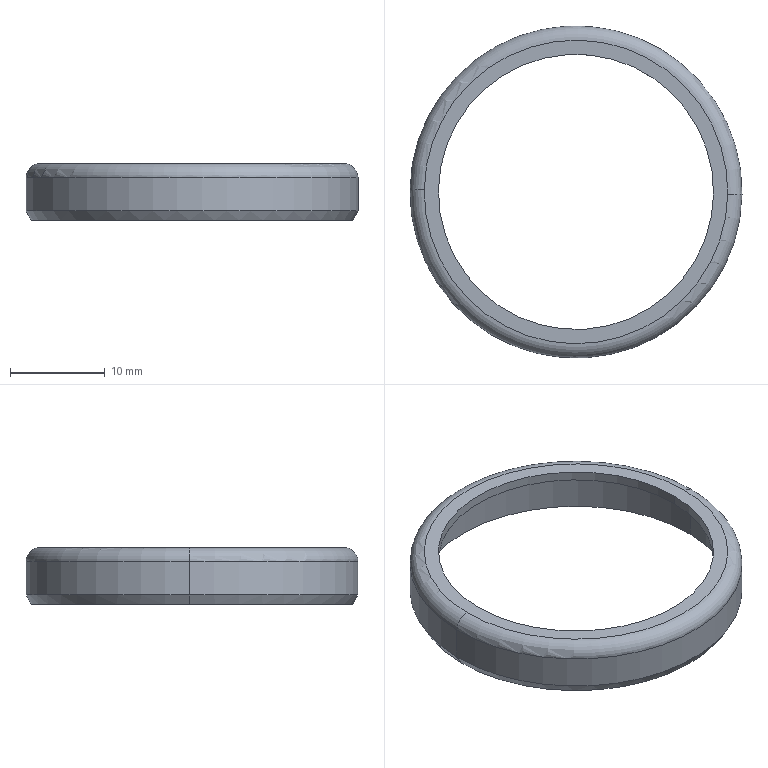Part | SolidWorks | features BaseBody 1 | 1 solid | 15 faces | box 35 x 35 x 6 mm | volume 627.231 mm3 | cylinder 6 | torus 4 | plane 3 | cone 2 | commonest cylinder face diameters 29 x2 33.5 x2 35 x2
STEP:
#1=CARTESIAN_POINT('',(-61.384,-49.853,89.25));
#2=VERTEX_POINT('',#1);
#3=CARTESIAN_POINT('',(-27.542,-50.354,89.25));
#4=VERTEX_POINT('',#3);
#5=CARTESIAN_POINT('',(-44.463,-50.104,89.25));
#6=DIRECTION('',(0.,0.,-1.));
#7=DIRECTION('',(-0.9999,0.01482,0.));
#8=AXIS2_PLACEMENT_3D('',#5,#6,#7);
#9=CIRCLE('',#8,16.923);
#10=EDGE_CURVE('',#2,#4,#9,.T.);
#11=ORIENTED_EDGE('',*,*,#10,.F.);
#12=CARTESIAN_POINT('',(-61.961,-49.845,90.25));
#13=VERTEX_POINT('',#12);
#14=CARTESIAN_POINT('',(-61.961,-49.845,90.25));
#15=DIRECTION('',(-0.4999,0.007408,0.866));
#16=VECTOR('',#15,1000.);
#17=LINE('',#14,#16);
#18=EDGE_CURVE('',#2,#13,#17,.T.);
#19=ORIENTED_EDGE('',*,*,#18,.T.);
#20=CARTESIAN_POINT('',(-26.965,-50.363,90.25));
#21=VERTEX_POINT('',#20);
#22=CARTESIAN_POINT('',(-44.463,-50.104,90.25));
#23=DIRECTION('',(0.,0.,-1.));
#24=DIRECTION('',(-0.9999,0.01482,0.));
#25=AXIS2_PLACEMENT_3D('',#22,#23,#24);
#26=CIRCLE('',#25,17.5);
#27=EDGE_CURVE('',#13,#21,#26,.T.);
#28=ORIENTED_EDGE('',*,*,#27,.T.);
#29=CARTESIAN_POINT('',(-26.965,-50.363,90.25));
#30=DIRECTION('',(0.4999,-0.007408,0.866));
#31=VECTOR('',#30,1000.);
#32=LINE('',#29,#31);
#33=EDGE_CURVE('',#4,#21,#32,.T.);
#34=ORIENTED_EDGE('',*,*,#33,.F.);
#35=EDGE_LOOP('',(#11,#19,#28,#34));
#36=FACE_OUTER_BOUND('',#35,.T.);
#37=CARTESIAN_POINT('',(-44.463,-50.104,90.25));
#38=DIRECTION('',(0.,0.,1.));
#39=DIRECTION('',(0.9999,-0.01482,0.));
#40=AXIS2_PLACEMENT_3D('',#37,#38,#39);
#41=CONICAL_SURFACE('',#40,17.5,0.5236);
#42=ADVANCED_FACE('',(#36),#41,.T.);
#43=CARTESIAN_POINT('',(-27.715,-50.352,93.75));
#44=VERTEX_POINT('',#43);
#45=CARTESIAN_POINT('',(-61.211,-49.856,93.75));
#46=VERTEX_POINT('',#45);
#47=CARTESIAN_POINT('',(-44.463,-50.104,93.75));
#48=DIRECTION('',(0.,0.,-1.));
#49=DIRECTION('',(-0.9999,0.01482,0.));
#50=AXIS2_PLACEMENT_3D('',#47,#48,#49);
#51=CIRCLE('',#50,16.75);
#52=EDGE_CURVE('',#44,#46,#51,.T.);
#53=ORIENTED_EDGE('',*,*,#52,.F.);
#54=CARTESIAN_POINT('',(-27.715,-50.352,89.25));
#55=VERTEX_POINT('',#54);
#56=CARTESIAN_POINT('',(-27.715,-50.352,89.25));
#57=DIRECTION('',(0.,0.,-1.));
#58=VECTOR('',#57,1000.);
#59=LINE('',#56,#58);
#60=EDGE_CURVE('',#44,#55,#59,.T.);
#61=ORIENTED_EDGE('',*,*,#60,.T.);
#62=CARTESIAN_POINT('',(-61.211,-49.856,89.25));
#63=VERTEX_POINT('',#62);
#64=CARTESIAN_POINT('',(-44.463,-50.104,89.25));
#65=DIRECTION('',(0.,0.,-1.));
#66=DIRECTION('',(-0.9999,0.01482,0.));
#67=AXIS2_PLACEMENT_3D('',#64,#65,#66);
#68=CIRCLE('',#67,16.75);
#69=EDGE_CURVE('',#55,#63,#68,.T.);
#70=ORIENTED_EDGE('',*,*,#69,.T.);
#71=CARTESIAN_POINT('',(-61.211,-49.856,89.25));
#72=DIRECTION('',(0.,0.,-1.));
#73=VECTOR('',#72,1000.);
#74=LINE('',#71,#73);
#75=EDGE_CURVE('',#46,#63,#74,.T.);
#76=ORIENTED_EDGE('',*,*,#75,.F.);
#77=EDGE_LOOP('',(#53,#61,#70,#76));
#78=FACE_OUTER_BOUND('',#77,.T.);
#79=CARTESIAN_POINT('',(-44.463,-50.104,89.25));
#80=DIRECTION('',(0.,0.,-1.));
#81=DIRECTION('',(-0.9999,0.01482,0.));
#82=AXIS2_PLACEMENT_3D('',#79,#80,#81);
#83=CYLINDRICAL_SURFACE('',#82,16.75);
#84=ADVANCED_FACE('',(#78),#83,.F.);
#85=CARTESIAN_POINT('',(-28.215,-50.345,94.25));
#86=VERTEX_POINT('',#85);
#87=CARTESIAN_POINT('',(-60.711,-49.863,94.25));
#88=VERTEX_POINT('',#87);
#89=CARTESIAN_POINT('',(-44.463,-50.104,94.25));
#90=DIRECTION('',(0.,0.,-1.));
#91=DIRECTION('',(-0.9999,0.01482,0.));
#92=AXIS2_PLACEMENT_3D('',#89,#90,#91);
#93=CIRCLE('',#92,16.25);
#94=EDGE_CURVE('',#86,#88,#93,.T.);
#95=ORIENTED_EDGE('',*,*,#94,.F.);
#96=CARTESIAN_POINT('',(-28.215,-50.345,93.75));
#97=DIRECTION('',(0.01482,0.9999,0.));
#98=DIRECTION('',(-0.9999,0.01482,0.));
#99=AXIS2_PLACEMENT_3D('',#96,#97,#98);
#100=CIRCLE('',#99,0.5);
#101=EDGE_CURVE('',#86,#44,#100,.T.);
#102=ORIENTED_EDGE('',*,*,#101,.T.);
#103=ORIENTED_EDGE('',*,*,#52,.T.);
#104=CARTESIAN_POINT('',(-60.711,-49.863,93.75));
#105=DIRECTION('',(-0.01482,-0.9999,0.));
#106=DIRECTION('',(0.9999,-0.01482,0.));
#107=AXIS2_PLACEMENT_3D('',#104,#105,#106);
#108=CIRCLE('',#107,0.5);
#109=EDGE_CURVE('',#88,#46,#108,.T.);
#110=ORIENTED_EDGE('',*,*,#109,.F.);
#111=EDGE_LOOP('',(#95,#102,#103,#110));
#112=FACE_OUTER_BOUND('',#111,.T.);
#113=CARTESIAN_POINT('',(-44.463,-50.104,93.75));
#114=DIRECTION('',(0.,0.,-1.));
#115=DIRECTION('',(-0.9999,0.01482,0.));
#116=AXIS2_PLACEMENT_3D('',#113,#114,#115);
#117=TOROIDAL_SURFACE('',#116,16.25,0.5);
#118=ADVANCED_FACE('',(#112),#117,.F.);
#119=CARTESIAN_POINT('',(-29.964,-50.319,95.25));
#120=VERTEX_POINT('',#119);
#121=CARTESIAN_POINT('',(-58.961,-49.889,95.25));
#122=VERTEX_POINT('',#121);
#123=CARTESIAN_POINT('',(-44.463,-50.104,95.25));
#124=DIRECTION('',(0.,0.,-1.));
#125=DIRECTION('',(-0.9999,0.01482,0.));
#126=AXIS2_PLACEMENT_3D('',#123,#124,#125);
#127=CIRCLE('',#126,14.5);
#128=EDGE_CURVE('',#120,#122,#127,.T.);
#129=ORIENTED_EDGE('',*,*,#128,.F.);
#130=CARTESIAN_POINT('',(-29.964,-50.319,94.25));
#131=VERTEX_POINT('',#130);
#132=CARTESIAN_POINT('',(-29.964,-50.319,89.25));
#133=DIRECTION('',(0.,0.,-1.));
#134=VECTOR('',#133,1000.);
#135=LINE('',#132,#134);
#136=EDGE_CURVE('',#120,#131,#135,.T.);
#137=ORIENTED_EDGE('',*,*,#136,.T.);
#138=CARTESIAN_POINT('',(-58.961,-49.889,94.25));
#139=VERTEX_POINT('',#138);
#140=CARTESIAN_POINT('',(-44.463,-50.104,94.25));
#141=DIRECTION('',(0.,0.,-1.));
#142=DIRECTION('',(-0.9999,0.01482,0.));
#143=AXIS2_PLACEMENT_3D('',#140,#141,#142);
#144=CIRCLE('',#143,14.5);
#145=EDGE_CURVE('',#131,#139,#144,.T.);
#146=ORIENTED_EDGE('',*,*,#145,.T.);
#147=CARTESIAN_POINT('',(-58.961,-49.889,89.25));
#148=DIRECTION('',(0.,0.,-1.));
#149=VECTOR('',#148,1000.);
#150=LINE('',#147,#149);
#151=EDGE_CURVE('',#122,#139,#150,.T.);
#152=ORIENTED_EDGE('',*,*,#151,.F.);
#153=EDGE_LOOP('',(#129,#137,#146,#152));
#154=FACE_OUTER_BOUND('',#153,.T.);
#155=CARTESIAN_POINT('',(-44.463,-50.104,89.25));
#156=DIRECTION('',(0.,0.,-1.));
#157=DIRECTION('',(-0.9999,0.01482,0.));
#158=AXIS2_PLACEMENT_3D('',#155,#156,#157);
#159=CYLINDRICAL_SURFACE('',#158,14.5);
#160=ADVANCED_FACE('',(#154),#159,.F.);
#161=CARTESIAN_POINT('',(-60.461,-49.867,95.25));
#162=VERTEX_POINT('',#161);
#163=CARTESIAN_POINT('',(-28.465,-50.341,95.25));
#164=VERTEX_POINT('',#163);
#165=CARTESIAN_POINT('',(-44.463,-50.104,95.25));
#166=DIRECTION('',(0.,0.,-1.));
#167=DIRECTION('',(-0.9999,0.01482,0.));
#168=AXIS2_PLACEMENT_3D('',#165,#166,#167);
#169=CIRCLE('',#168,16.);
#170=EDGE_CURVE('',#162,#164,#169,.T.);
#171=ORIENTED_EDGE('',*,*,#170,.T.);
#172=CARTESIAN_POINT('',(-26.965,-50.363,93.75));
#173=VERTEX_POINT('',#172);
#174=CARTESIAN_POINT('',(-28.465,-50.341,93.75));
#175=DIRECTION('',(0.01482,0.9999,0.));
#176=DIRECTION('',(-0.9999,0.01482,0.));
#177=AXIS2_PLACEMENT_3D('',#174,#175,#176);
#178=CIRCLE('',#177,1.5);
#179=EDGE_CURVE('',#164,#173,#178,.T.);
#180=ORIENTED_EDGE('',*,*,#179,.T.);
#181=CARTESIAN_POINT('',(-61.961,-49.845,93.75));
#182=VERTEX_POINT('',#181);
#183=CARTESIAN_POINT('',(-44.463,-50.104,93.75));
#184=DIRECTION('',(0.,0.,-1.));
#185=DIRECTION('',(-0.9999,0.01482,0.));
#186=AXIS2_PLACEMENT_3D('',#183,#184,#185);
#187=CIRCLE('',#186,17.5);
#188=EDGE_CURVE('',#182,#173,#187,.T.);
#189=ORIENTED_EDGE('',*,*,#188,.F.);
#190=CARTESIAN_POINT('',(-60.461,-49.867,93.75));
#191=DIRECTION('',(-0.01482,-0.9999,0.));
#192=DIRECTION('',(0.9999,-0.01482,0.));
#193=AXIS2_PLACEMENT_3D('',#190,#191,#192);
#194=CIRCLE('',#193,1.5);
#195=EDGE_CURVE('',#162,#182,#194,.T.);
#196=ORIENTED_EDGE('',*,*,#195,.F.);
#197=EDGE_LOOP('',(#171,#180,#189,#196));
#198=FACE_OUTER_BOUND('',#197,.T.);
#199=CARTESIAN_POINT('',(-44.463,-50.104,93.75));
#200=DIRECTION('',(0.,0.,-1.));
#201=DIRECTION('',(-0.9999,0.01482,0.));
#202=AXIS2_PLACEMENT_3D('',#199,#200,#201);
#203=TOROIDAL_SURFACE('',#202,16.,1.5);
#204=ADVANCED_FACE('',(#198),#203,.T.);
#205=ORIENTED_EDGE('',*,*,#188,.T.);
#206=CARTESIAN_POINT('',(-26.965,-50.363,89.25));
#207=DIRECTION('',(0.,0.,-1.));
#208=VECTOR('',#207,1000.);
#209=LINE('',#206,#208);
#210=EDGE_CURVE('',#173,#21,#209,.T.);
#211=ORIENTED_EDGE('',*,*,#210,.T.);
#212=ORIENTED_EDGE('',*,*,#27,.F.);
#213=CARTESIAN_POINT('',(-61.961,-49.845,89.25));
#214=DIRECTION('',(0.,0.,-1.));
#215=VECTOR('',#214,1000.);
#216=LINE('',#213,#215);
#217=EDGE_CURVE('',#182,#13,#216,.T.);
#218=ORIENTED_EDGE('',*,*,#217,.F.);
#219=EDGE_LOOP('',(#205,#211,#212,#218));
#220=FACE_OUTER_BOUND('',#219,.T.);
#221=CARTESIAN_POINT('',(-44.463,-50.104,89.25));
#222=DIRECTION('',(0.,0.,-1.));
#223=DIRECTION('',(-0.9999,0.01482,0.));
#224=AXIS2_PLACEMENT_3D('',#221,#222,#223);
#225=CYLINDRICAL_SURFACE('',#224,17.5);
#226=ADVANCED_FACE('',(#220),#225,.T.);
#227=ORIENTED_EDGE('',*,*,#210,.F.);
#228=CARTESIAN_POINT('',(-44.463,-50.104,93.75));
#229=DIRECTION('',(0.,0.,-1.));
#230=DIRECTION('',(-0.9999,0.01482,0.));
#231=AXIS2_PLACEMENT_3D('',#228,#229,#230);
#232=CIRCLE('',#231,17.5);
#233=EDGE_CURVE('',#173,#182,#232,.T.);
#234=ORIENTED_EDGE('',*,*,#233,.T.);
#235=ORIENTED_EDGE('',*,*,#217,.T.);
#236=CARTESIAN_POINT('',(-44.463,-50.104,90.25));
#237=DIRECTION('',(0.,0.,-1.));
#238=DIRECTION('',(-0.9999,0.01482,0.));
#239=AXIS2_PLACEMENT_3D('',#236,#237,#238);
#240=CIRCLE('',#239,17.5);
#241=EDGE_CURVE('',#21,#13,#240,.T.);
#242=ORIENTED_EDGE('',*,*,#241,.F.);
#243=EDGE_LOOP('',(#227,#234,#235,#242));
#244=FACE_OUTER_BOUND('',#243,.T.);
#245=CARTESIAN_POINT('',(-44.463,-50.104,89.25));
#246=DIRECTION('',(0.,0.,-1.));
#247=DIRECTION('',(-0.9999,0.01482,0.));
#248=AXIS2_PLACEMENT_3D('',#245,#246,#247);
#249=CYLINDRICAL_SURFACE('',#248,17.5);
#250=ADVANCED_FACE('',(#244),#249,.T.);
#251=ORIENTED_EDGE('',*,*,#179,.F.);
#252=CARTESIAN_POINT('',(-44.463,-50.104,95.25));
#253=DIRECTION('',(0.,0.,-1.));
#254=DIRECTION('',(-0.9999,0.01482,0.));
#255=AXIS2_PLACEMENT_3D('',#252,#253,#254);
#256=CIRCLE('',#255,16.);
#257=EDGE_CURVE('',#164,#162,#256,.T.);
#258=ORIENTED_EDGE('',*,*,#257,.T.);
#259=ORIENTED_EDGE('',*,*,#195,.T.);
#260=ORIENTED_EDGE('',*,*,#233,.F.);
#261=EDGE_LOOP('',(#251,#258,#259,#260));
#262=FACE_OUTER_BOUND('',#261,.T.);
#263=CARTESIAN_POINT('',(-44.463,-50.104,93.75));
#264=DIRECTION('',(0.,0.,-1.));
#265=DIRECTION('',(-0.9999,0.01482,0.));
#266=AXIS2_PLACEMENT_3D('',#263,#264,#265);
#267=TOROIDAL_SURFACE('',#266,16.,1.5);
#268=ADVANCED_FACE('',(#262),#267,.T.);
#269=CARTESIAN_POINT('',(-44.463,-50.104,95.25));
#270=DIRECTION('',(0.,0.,-1.));
#271=DIRECTION('',(-0.9999,0.01482,0.));
#272=AXIS2_PLACEMENT_3D('',#269,#270,#271);
#273=CIRCLE('',#272,14.5);
#274=EDGE_CURVE('',#122,#120,#273,.T.);
#275=ORIENTED_EDGE('',*,*,#274,.T.);
#276=ORIENTED_EDGE('',*,*,#128,.T.);
#277=EDGE_LOOP('',(#275,#276));
#278=FACE_BOUND('',#277,.T.);
#279=ORIENTED_EDGE('',*,*,#170,.F.);
#280=ORIENTED_EDGE('',*,*,#257,.F.);
#281=EDGE_LOOP('',(#279,#280));
#282=FACE_OUTER_BOUND('',#281,.T.);
#283=CARTESIAN_POINT('',(-44.226,-34.106,95.25));
#284=DIRECTION('',(0.,0.,-1.));
#285=DIRECTION('',(-1.,0.,0.));
#286=AXIS2_PLACEMENT_3D('',#283,#284,#285);
#287=PLANE('',#286);
#288=ADVANCED_FACE('',(#278,#282),#287,.F.);
#289=ORIENTED_EDGE('',*,*,#136,.F.);
#290=ORIENTED_EDGE('',*,*,#274,.F.);
#291=ORIENTED_EDGE('',*,*,#151,.T.);
#292=CARTESIAN_POINT('',(-44.463,-50.104,94.25));
#293=DIRECTION('',(0.,0.,-1.));
#294=DIRECTION('',(-0.9999,0.01482,0.));
#295=AXIS2_PLACEMENT_3D('',#292,#293,#294);
#296=CIRCLE('',#295,14.5);
#297=EDGE_CURVE('',#139,#131,#296,.T.);
#298=ORIENTED_EDGE('',*,*,#297,.T.);
#299=EDGE_LOOP('',(#289,#290,#291,#298));
#300=FACE_OUTER_BOUND('',#299,.T.);
#301=CARTESIAN_POINT('',(-44.463,-50.104,89.25));
#302=DIRECTION('',(0.,0.,-1.));
#303=DIRECTION('',(-0.9999,0.01482,0.));
#304=AXIS2_PLACEMENT_3D('',#301,#302,#303);
#305=CYLINDRICAL_SURFACE('',#304,14.5);
#306=ADVANCED_FACE('',(#300),#305,.F.);
#307=CARTESIAN_POINT('',(-44.463,-50.104,94.25));
#308=DIRECTION('',(0.,0.,-1.));
#309=DIRECTION('',(-0.9999,0.01482,0.));
#310=AXIS2_PLACEMENT_3D('',#307,#308,#309);
#311=CIRCLE('',#310,16.25);
#312=EDGE_CURVE('',#88,#86,#311,.T.);
#313=ORIENTED_EDGE('',*,*,#312,.T.);
#314=ORIENTED_EDGE('',*,*,#94,.T.);
#315=EDGE_LOOP('',(#313,#314));
#316=FACE_OUTER_BOUND('',#315,.T.);
#317=ORIENTED_EDGE('',*,*,#297,.F.);
#318=ORIENTED_EDGE('',*,*,#145,.F.);
#319=EDGE_LOOP('',(#317,#318));
#320=FACE_BOUND('',#319,.T.);
#321=CARTESIAN_POINT('',(-44.248,-35.605,94.25));
#322=DIRECTION('',(0.,0.,1.));
#323=DIRECTION('',(1.,0.,0.));
#324=AXIS2_PLACEMENT_3D('',#321,#322,#323);
#325=PLANE('',#324);
#326=ADVANCED_FACE('',(#316,#320),#325,.F.);
#327=ORIENTED_EDGE('',*,*,#101,.F.);
#328=ORIENTED_EDGE('',*,*,#312,.F.);
#329=ORIENTED_EDGE('',*,*,#109,.T.);
#330=CARTESIAN_POINT('',(-44.463,-50.104,93.75));
#331=DIRECTION('',(0.,0.,-1.));
#332=DIRECTION('',(-0.9999,0.01482,0.));
#333=AXIS2_PLACEMENT_3D('',#330,#331,#332);
#334=CIRCLE('',#333,16.75);
#335=EDGE_CURVE('',#46,#44,#334,.T.);
#336=ORIENTED_EDGE('',*,*,#335,.T.);
#337=EDGE_LOOP('',(#327,#328,#329,#336));
#338=FACE_OUTER_BOUND('',#337,.T.);
#339=CARTESIAN_POINT('',(-44.463,-50.104,93.75));
#340=DIRECTION('',(0.,0.,-1.));
#341=DIRECTION('',(-0.9999,0.01482,0.));
#342=AXIS2_PLACEMENT_3D('',#339,#340,#341);
#343=TOROIDAL_SURFACE('',#342,16.25,0.5);
#344=ADVANCED_FACE('',(#338),#343,.F.);
#345=ORIENTED_EDGE('',*,*,#60,.F.);
#346=ORIENTED_EDGE('',*,*,#335,.F.);
#347=ORIENTED_EDGE('',*,*,#75,.T.);
#348=CARTESIAN_POINT('',(-44.463,-50.104,89.25));
#349=DIRECTION('',(0.,0.,-1.));
#350=DIRECTION('',(-0.9999,0.01482,0.));
#351=AXIS2_PLACEMENT_3D('',#348,#349,#350);
#352=CIRCLE('',#351,16.75);
#353=EDGE_CURVE('',#63,#55,#352,.T.);
#354=ORIENTED_EDGE('',*,*,#353,.T.);
#355=EDGE_LOOP('',(#345,#346,#347,#354));
#356=FACE_OUTER_BOUND('',#355,.T.);
#357=CARTESIAN_POINT('',(-44.463,-50.104,89.25));
#358=DIRECTION('',(0.,0.,-1.));
#359=DIRECTION('',(-0.9999,0.01482,0.));
#360=AXIS2_PLACEMENT_3D('',#357,#358,#359);
#361=CYLINDRICAL_SURFACE('',#360,16.75);
#362=ADVANCED_FACE('',(#356),#361,.F.);
#363=CARTESIAN_POINT('',(-44.463,-50.104,89.25));
#364=DIRECTION('',(0.,0.,-1.));
#365=DIRECTION('',(-0.9999,0.01482,0.));
#366=AXIS2_PLACEMENT_3D('',#363,#364,#365);
#367=CIRCLE('',#366,16.923);
#368=EDGE_CURVE('',#4,#2,#367,.T.);
#369=ORIENTED_EDGE('',*,*,#368,.T.);
#370=ORIENTED_EDGE('',*,*,#10,.T.);
#371=EDGE_LOOP('',(#369,#370));
#372=FACE_OUTER_BOUND('',#371,.T.);
#373=ORIENTED_EDGE('',*,*,#353,.F.);
#374=ORIENTED_EDGE('',*,*,#69,.F.);
#375=EDGE_LOOP('',(#373,#374));
#376=FACE_BOUND('',#375,.T.);
#377=CARTESIAN_POINT('',(-44.215,-33.356,89.25));
#378=DIRECTION('',(0.,0.,1.));
#379=DIRECTION('',(1.,0.,0.));
#380=AXIS2_PLACEMENT_3D('',#377,#378,#379);
#381=PLANE('',#380);
#382=ADVANCED_FACE('',(#372,#376),#381,.F.);
#383=ORIENTED_EDGE('',*,*,#18,.F.);
#384=ORIENTED_EDGE('',*,*,#368,.F.);
#385=ORIENTED_EDGE('',*,*,#33,.T.);
#386=ORIENTED_EDGE('',*,*,#241,.T.);
#387=EDGE_LOOP('',(#383,#384,#385,#386));
#388=FACE_OUTER_BOUND('',#387,.T.);
#389=CARTESIAN_POINT('',(-44.463,-50.104,90.25));
#390=DIRECTION('',(0.,0.,1.));
#391=DIRECTION('',(0.9999,-0.01482,0.));
#392=AXIS2_PLACEMENT_3D('',#389,#390,#391);
#393=CONICAL_SURFACE('',#392,17.5,0.5236);
#394=ADVANCED_FACE('',(#388),#393,.T.);
#395=CLOSED_SHELL('',(#42,#84,#118,#160,#204,#226,#250,#268,#288,#306,#326,#344,#362,#382,#394));
#396=MANIFOLD_SOLID_BREP('',#395);
#397=CARTESIAN_POINT('',(0.,0.,0.));
#398=DIRECTION('',(0.,0.,1.));
#399=DIRECTION('',(1.,0.,0.));
#400=AXIS2_PLACEMENT_3D('',#397,#398,#399);
#401=(LENGTH_UNIT()NAMED_UNIT(*)SI_UNIT(.MILLI.,.METRE.));
#402=UNCERTAINTY_MEASURE_WITH_UNIT(LENGTH_MEASURE(0.00001),#401,'','');
#403=(NAMED_UNIT(*)PLANE_ANGLE_UNIT()SI_UNIT($,.RADIAN.));
#404=(NAMED_UNIT(*)SI_UNIT($,.STERADIAN.)SOLID_ANGLE_UNIT());
#405=(GEOMETRIC_REPRESENTATION_CONTEXT(3)GLOBAL_UNCERTAINTY_ASSIGNED_CONTEXT((#402))GLOBAL_UNIT_ASSIGNED_CONTEXT((#401,#403,#404))REPRESENTATION_CONTEXT('',''));
#406=ADVANCED_BREP_SHAPE_REPRESENTATION('',(#396,#400),#405);